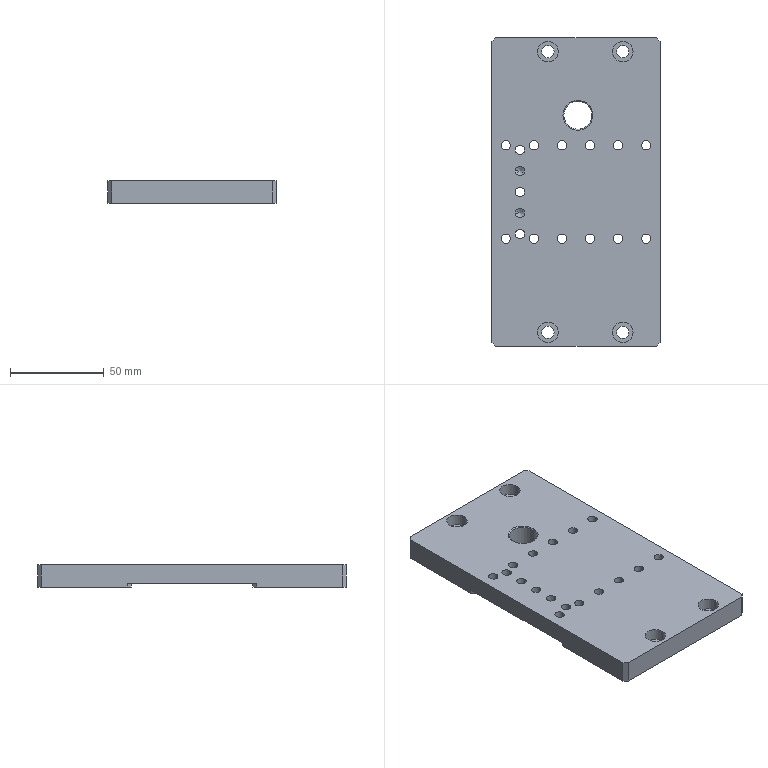NC program | NX | posted with a generic post | part box 90 x 165 x 12 mm
Whole program:
N10 G17 G21 G94 G90
(DRILLING , TOOL : D6A45)
N12 T01 M6
N14 G54
N16 G17 G0 G90 X157.5 Y60. S9500 M3
N18 G43 Z30. H1
N20 G94 G81 G98 Z-1. F250. R3.
N22 Y20.
N24 X107.5 Y7.5
N26 Y22.5
N28 Y37.5
N30 X123.5 Y44.
N32 X107.5 Y52.5
N34 Y67.5
N36 X105. Y75.
N38 X107.5 Y82.5
N40 X93.75 Y75.
N42 X82.5
N44 X71.25
N46 X57.5 Y82.5
N48 X60. Y75.
N50 X57.5 Y67.5
N52 Y52.5
N54 Y37.5
N56 Y22.5
N58 Y7.5
N60 X7.5 Y20.
N62 Y60.
N64 G80
N66 G0 X7.5 Y60. Z30.
N68 M5
(DRILLING_COPY , TOOL : 6.6ZT)
N70 T10 M6
N72 G54
N74 G17 G0 G90 X7.5 Y20. S2000 M3
N76 G43 Z30. H10
N78 G94 G83 G98 Z-14.483 F250. Q2. R3.
N80 Y60.
N82 X157.5
N84 Y20.
N86 G80
N88 G0 X157.5 Y20. Z30.
N90 M5
(DRILLING_COPY_COPY , TOOL : 5.0ZT)
N92 T17 M6
N94 G54
N96 G17 G0 G90 X107.5 Y7.5 S2000 M3
N98 G43 Z30. H17
N100 G94 G83 G98 Z-14.002 F250. Q2. R3.
N102 Y22.5
N104 Y37.5
N106 Y52.5
N108 Y67.5
N110 X105. Y75.
N112 X107.5 Y82.5
N114 X82.5 Y75.
N116 X57.5 Y82.5
N118 X60. Y75.
N120 X57.5 Y67.5
N122 Y52.5
N124 Y37.5
N126 Y22.5
N128 Y7.5
N130 G80
N132 G0 X57.5 Y7.5 Z30.
N134 M5
(ZLEVEL_PROFILE , TOOL : D10)
N136 T15 M6
N138 G54
N140 G17 G0 G90 X163.037 Y99.812 S9500 M3
N142 G43 Z30. H15
N144 Z2.
N146 G94 G1 Z-1. F1000.
N148 X162.629 Y98.29
N150 G3 X162.888 Y97.324 R1.
N152 G1 X167.249 Y92.964 F3000.
N154 X168.606 Y91.606
N156 G2 X170.1 Y88. R5.1
N158 G1 Y2.
N160 G2 X168.606 Y-1.606 R5.1
N162 G1 X166.674 Y-3.539
N164 G2 X166.056 Y-4.083 R6.519
N166 G1 X166.047 Y-4.165
N168 X162.888 Y-7.324
N170 G3 X162.629 Y-8.29 R1.
N172 G1 X163.037 Y-9.812
N174 Z2.
N176 G0 Z1.
N178 G1 Z-2. F1000.
N180 X162.629 Y-8.29
N182 G2 X162.888 Y-7.324 R1.
N184 G1 X166.047 Y-4.165 F3000.
N186 X166.056 Y-4.083
N188 G3 X166.674 Y-3.539 R6.519
N190 G1 X168.606 Y-1.606
N192 G3 X170.1 Y2. R5.1
N194 G1 Y88.
N196 G3 X168.606 Y91.606 R5.1
N198 G1 X167.249 Y92.964
N200 X162.888 Y97.324
N202 G2 X162.629 Y98.29 R1.
N204 G1 X163.037 Y99.812
N206 Z1.
N208 G0 Z0.
N210 G1 Z-3. F1000.
N212 X162.629 Y98.29
N214 G3 X162.888 Y97.324 R1.
N216 G1 X167.249 Y92.964 F3000.
N218 X168.606 Y91.606
N220 G2 X170.1 Y88. R5.1
N222 G1 Y2.
N224 G2 X168.606 Y-1.606 R5.1
N226 G1 X166.674 Y-3.539
N228 G2 X166.056 Y-4.083 R6.519
N230 G1 X166.047 Y-4.165
N232 X162.888 Y-7.324
N234 G3 X162.629 Y-8.29 R1.
N236 G1 X163.037 Y-9.812
N238 Z0.
N240 G0 Z-1.
N242 G1 Z-4. F1000.
N244 X162.629 Y-8.29
N246 G2 X162.888 Y-7.324 R1.
N248 G1 X166.047 Y-4.165 F3000.
N250 X166.056 Y-4.083
N252 G3 X166.674 Y-3.539 R6.519
N254 G1 X168.606 Y-1.606
N256 G3 X170.1 Y2. R5.1
N258 G1 Y88.
N260 G3 X168.606 Y91.606 R5.1
N262 G1 X167.249 Y92.964
N264 X162.888 Y97.324
N266 G2 X162.629 Y98.29 R1.
N268 G1 X163.037 Y99.812
N270 Z-1.
N272 G0 Z-2.
N274 G1 Z-5. F1000.
N276 X162.629 Y98.29
N278 G3 X162.888 Y97.324 R1.
N280 G1 X167.249 Y92.964 F3000.
N282 X168.606 Y91.606
N284 G2 X170.1 Y88. R5.1
N286 G1 Y2.
N288 G2 X168.606 Y-1.606 R5.1
N290 G1 X166.674 Y-3.539
N292 G2 X166.056 Y-4.083 R6.519
N294 G1 X166.047 Y-4.165
N296 X162.888 Y-7.324
N298 G3 X162.629 Y-8.29 R1.
N300 G1 X163.037 Y-9.812
N302 Z-2.
N304 G0 Z-3.
N306 G1 Z-6. F1000.
N308 X162.629 Y-8.29
N310 G2 X162.888 Y-7.324 R1.
N312 G1 X166.047 Y-4.165 F3000.
N314 X166.056 Y-4.083
N316 G3 X166.674 Y-3.539 R6.519
N318 G1 X168.606 Y-1.606
N320 G3 X170.1 Y2. R5.1
N322 G1 Y88.
N324 G3 X168.606 Y91.606 R5.1
N326 G1 X167.249 Y92.964
N328 X162.888 Y97.324
N330 G2 X162.629 Y98.29 R1.
N332 G1 X163.037 Y99.812
N334 Z-3.
N336 G0 Z-4.
N338 G1 Z-7. F1000.
N340 X162.629 Y98.29
N342 G3 X162.888 Y97.324 R1.
N344 G1 X167.249 Y92.964 F3000.
N346 X168.606 Y91.606
N348 G2 X170.1 Y88. R5.1
N350 G1 Y2.
N352 G2 X168.606 Y-1.606 R5.1
N354 G1 X166.674 Y-3.539
N356 G2 X166.056 Y-4.083 R6.519
N358 G1 X166.047 Y-4.165
N360 X162.888 Y-7.324
N362 G3 X162.629 Y-8.29 R1.
N364 G1 X163.037 Y-9.812
N366 Z-4.
N368 G0 Z-5.
N370 G1 Z-8. F1000.
N372 X162.629 Y-8.29
N374 G2 X162.888 Y-7.324 R1.
N376 G1 X166.047 Y-4.165 F3000.
N378 X166.056 Y-4.083
N380 G3 X166.674 Y-3.539 R6.519
N382 G1 X168.606 Y-1.606
N384 G3 X170.1 Y2. R5.1
N386 G1 Y88.
N388 G3 X168.606 Y91.606 R5.1
N390 G1 X167.249 Y92.964
N392 X162.888 Y97.324
N394 G2 X162.629 Y98.29 R1.
N396 G1 X163.037 Y99.812
N398 Z-5.
N400 G0 Z-6.
N402 G1 Z-9. F1000.
N404 X162.629 Y98.29
N406 G3 X162.888 Y97.324 R1.
N408 G1 X167.249 Y92.964 F3000.
N410 X168.606 Y91.606
N412 G2 X170.1 Y88. R5.1
N414 G1 Y2.
N416 G2 X168.606 Y-1.606 R5.1
N418 G1 X166.674 Y-3.539
N420 G2 X166.056 Y-4.083 R6.519
N422 G1 X166.047 Y-4.165
N424 X162.888 Y-7.324
N426 G3 X162.629 Y-8.29 R1.
N428 G1 X163.037 Y-9.812
N430 Z-6.
N432 G0 Z-7.
N434 G1 Z-10. F1000.
N436 X162.629 Y-8.29
N438 G2 X162.888 Y-7.324 R1.
N440 G1 X166.047 Y-4.165 F3000.
N442 X166.056 Y-4.083
N444 G3 X166.674 Y-3.539 R6.519
N446 G1 X168.606 Y-1.606
N448 G3 X170.1 Y2. R5.1
N450 G1 Y88.
N452 G3 X168.606 Y91.606 R5.1
N454 G1 X167.249 Y92.964
N456 X162.888 Y97.324
N458 G2 X162.629 Y98.29 R1.
N460 G1 X163.037 Y99.812
N462 Z-7.
N464 G0 Z-8.
N466 G1 Z-11. F1000.
N468 X162.629 Y98.29
N470 G3 X162.888 Y97.324 R1.
N472 G1 X167.249 Y92.964 F3000.
N474 X168.606 Y91.606
N476 G2 X170.1 Y88. R5.1
N478 G1 Y2.
N480 G2 X168.606 Y-1.606 R5.1
N482 G1 X166.674 Y-3.539
N484 G2 X166.056 Y-4.083 R6.519
N486 G1 X166.047 Y-4.165
N488 X162.888 Y-7.324
N490 G3 X162.629 Y-8.29 R1.
N492 G1 X163.037 Y-9.812
N494 Z-8.
N496 G0 Z-9.
N498 G1 Z-12. F1000.
N500 X162.629 Y-8.29
N502 G2 X162.888 Y-7.324 R1.
N504 G1 X166.047 Y-4.165 F3000.
N506 X166.056 Y-4.083
N508 G3 X166.674 Y-3.539 R6.519
N510 G1 X168.606 Y-1.606
N512 G3 X170.1 Y2. R5.1
N514 G1 Y88.
N516 G3 X168.606 Y91.606 R5.1
N518 G1 X167.249 Y92.964
N520 X162.888 Y97.324
N522 G2 X162.629 Y98.29 R1.
N524 G1 X163.037 Y99.812
N526 Z-9.
N528 G0 Z58.5
N530 X2.066 Y-9.873
N532 Z2.
N534 G1 Z-1. F1000.
N536 X2.465 Y-8.384
N538 G3 X2.206 Y-7.418 R1.
N540 G1 X-1.627 Y-3.585 F3000.
N542 X-2.9 Y-2.308
N544 X-3.018 Y-2.111
N546 G2 X-5.1 Y2. R5.1
N548 G1 Y88.
N550 G2 X-3.606 Y91.606 R5.1
N552 G1 X-1.606 Y93.606
N554 X2.106 Y97.318
N556 G3 X2.365 Y98.284 R1.
N558 G1 X1.957 Y99.805
N560 Z2.
N562 G0 Z1.
N564 G1 Z-2. F1000.
N566 X2.365 Y98.284
N568 G2 X2.106 Y97.318 R1.
N570 G1 X-1.606 Y93.606 F3000.
N572 X-3.606 Y91.606
N574 G3 X-5.1 Y88. R5.1
N576 G1 Y2.
N578 G3 X-3.018 Y-2.111 R5.1
N580 G1 X-2.9 Y-2.308
N582 X-1.627 Y-3.585
N584 X2.206 Y-7.418
N586 G2 X2.465 Y-8.384 R1.
N588 G1 X2.066 Y-9.873
N590 Z1.
N592 G0 Z0.
N594 G1 Z-3. F1000.
N596 X2.465 Y-8.384
N598 G3 X2.206 Y-7.418 R1.
N600 G1 X-1.627 Y-3.585 F3000.
N602 X-2.9 Y-2.308
N604 X-3.018 Y-2.111
N606 G2 X-5.1 Y2. R5.1
N608 G1 Y88.
N610 G2 X-3.606 Y91.606 R5.1
N612 G1 X-1.606 Y93.606
N614 X2.106 Y97.318
N616 G3 X2.365 Y98.284 R1.
N618 G1 X1.957 Y99.805
N620 Z0.
N622 G0 Z-1.
N624 G1 Z-4. F1000.
N626 X2.365 Y98.284
N628 G2 X2.106 Y97.318 R1.
N630 G1 X-1.606 Y93.606 F3000.
N632 X-3.606 Y91.606
N634 G3 X-5.1 Y88. R5.1
N636 G1 Y2.
N638 G3 X-3.018 Y-2.111 R5.1
N640 G1 X-2.9 Y-2.308
N642 X-1.627 Y-3.585
N644 X2.206 Y-7.418
N646 G2 X2.465 Y-8.384 R1.
N648 G1 X2.066 Y-9.873
N650 Z-1.
N652 G0 Z-2.
N654 G1 Z-5. F1000.
N656 X2.465 Y-8.384
N658 G3 X2.206 Y-7.418 R1.
N660 G1 X-1.627 Y-3.585 F3000.
N662 X-2.9 Y-2.308
N664 X-3.018 Y-2.111
N666 G2 X-5.1 Y2. R5.1
N668 G1 Y88.
N670 G2 X-3.606 Y91.606 R5.1
N672 G1 X-1.606 Y93.606
N674 X2.106 Y97.318
N676 G3 X2.365 Y98.284 R1.
N678 G1 X1.957 Y99.805
N680 Z-2.
N682 G0 Z-3.
N684 G1 Z-6. F1000.
N686 X2.365 Y98.284
N688 G2 X2.106 Y97.318 R1.
N690 G1 X-1.606 Y93.606 F3000.
N692 X-3.606 Y91.606
N694 G3 X-5.1 Y88. R5.1
N696 G1 Y2.
N698 G3 X-3.018 Y-2.111 R5.1
N700 G1 X-2.9 Y-2.308
N702 X-1.627 Y-3.585
N704 X2.206 Y-7.418
N706 G2 X2.465 Y-8.384 R1.
N708 G1 X2.066 Y-9.873
N710 Z-3.
N712 G0 Z-4.
N714 G1 Z-7. F1000.
N716 X2.465 Y-8.384
N718 G3 X2.206 Y-7.418 R1.
N720 G1 X-1.627 Y-3.585 F3000.
N722 X-2.9 Y-2.308
N724 X-3.018 Y-2.111
N726 G2 X-5.1 Y2. R5.1
N728 G1 Y88.
N730 G2 X-3.606 Y91.606 R5.1
N732 G1 X-1.606 Y93.606
N734 X2.106 Y97.318
N736 G3 X2.365 Y98.284 R1.
N738 G1 X1.957 Y99.805
N740 Z-4.
N742 G0 Z-5.
N744 G1 Z-8. F1000.
N746 X2.365 Y98.284
N748 G2 X2.106 Y97.318 R1.
N750 G1 X-1.606 Y93.606 F3000.
N752 X-3.606 Y91.606
N754 G3 X-5.1 Y88. R5.1
N756 G1 Y2.
N758 G3 X-3.018 Y-2.111 R5.1
N760 G1 X-2.9 Y-2.308
N762 X-1.627 Y-3.585
N764 X2.206 Y-7.418
N766 G2 X2.465 Y-8.384 R1.
N768 G1 X2.066 Y-9.873
N770 Z-5.
N772 G0 Z-6.
N774 G1 Z-9. F1000.
N776 X2.465 Y-8.384
N778 G3 X2.206 Y-7.418 R1.
N780 G1 X-1.627 Y-3.585 F3000.
N782 X-2.9 Y-2.308
N784 X-3.018 Y-2.111
N786 G2 X-5.1 Y2. R5.1
N788 G1 Y88.
N790 G2 X-3.606 Y91.606 R5.1
N792 G1 X-1.606 Y93.606
N794 X2.106 Y97.318
N796 G3 X2.365 Y98.284 R1.
N798 G1 X1.957 Y99.805
N800 Z-6.
N802 G0 Z-7.
N804 G1 Z-10. F1000.
N806 X2.365 Y98.284
N808 G2 X2.106 Y97.318 R1.
N810 G1 X-1.606 Y93.606 F3000.
N812 X-3.606 Y91.606
N814 G3 X-5.1 Y88. R5.1
N816 G1 Y2.
N818 G3 X-3.018 Y-2.111 R5.1
N820 G1 X-2.9 Y-2.308
N822 X-1.627 Y-3.585
N824 X2.206 Y-7.418
N826 G2 X2.465 Y-8.384 R1.
N828 G1 X2.066 Y-9.873
N830 Z-7.
N832 G0 Z-8.
N834 G1 Z-11. F1000.
N836 X2.465 Y-8.384
N838 G3 X2.206 Y-7.418 R1.
N840 G1 X-1.627 Y-3.585 F3000.
N842 X-2.9 Y-2.308
N844 X-3.018 Y-2.111
N846 G2 X-5.1 Y2. R5.1
N848 G1 Y88.
N850 G2 X-3.606 Y91.606 R5.1
N852 G1 X-1.606 Y93.606
N854 X2.106 Y97.318
N856 G3 X2.365 Y98.284 R1.
N858 G1 X1.957 Y99.805
N860 Z-8.
N862 G0 Z-9.
N864 G1 Z-12. F1000.
N866 X2.365 Y98.284
N868 G2 X2.106 Y97.318 R1.
N870 G1 X-1.606 Y93.606 F3000.
N872 X-3.606 Y91.606
N874 G3 X-5.1 Y88. R5.1
N876 G1 Y2.
N878 G3 X-3.018 Y-2.111 R5.1
N880 G1 X-2.9 Y-2.308
N882 X-1.627 Y-3.585
N884 X2.206 Y-7.418
N886 G2 X2.465 Y-8.384 R1.
N888 G1 X2.066 Y-9.873
N890 Z-9.
N892 G0 Z30.
N894 M5
(HOLE_MILLING , TOOL : D6)
N896 T12 M6
N898 G54
N900 G17 G0 G90 X7.5 Y60. S9500 M3
N902 G43 Z30. H12
N904 Z0.5
N906 G94 G3 X6.25 Y58.75 R1.25 F1500.
N908 X7.5 Y57.5 R1.25
N910 X7.5 Y57.5 Z-0.1 I0. J2.5
N912 X7.5 Y57.5 Z-0.7 I0. J2.5
N914 X7.5 Y57.5 Z-1.3 I0. J2.5
N916 X7.5 Y57.5 Z-1.9 I0. J2.5
N918 X7.5 Y57.5 Z-2.5 I0. J2.5
N920 X7.5 Y57.5 Z-3.1 I0. J2.5
N922 X7.5 Y57.5 Z-3.7 I0. J2.5
N924 X7.5 Y57.5 Z-4.3 I0. J2.5
N926 X7.5 Y57.5 Z-4.9 I0. J2.5
N928 X7.5 Y57.5 Z-5.5 I0. J2.5
N930 X7.5 Y57.5 Z-6.1 I0. J2.5
N932 X7.5 Y62.5 Z-6.4 I0. J2.5
N934 X5. Y60. R2.5
N936 X7.5 Y62.5 R-2.5
N938 X6.25 Y61.25 R1.25
N940 X7.5 Y60. R1.25
N942 G0 Z30.
N944 Y20.
N946 Z0.5
N948 G3 X6.25 Y18.75 R1.25
N950 X7.5 Y17.5 R1.25
N952 X7.5 Y17.5 Z-0.1 I0. J2.5
N954 X7.5 Y17.5 Z-0.7 I0. J2.5
N956 X7.5 Y17.5 Z-1.3 I0. J2.5
N958 X7.5 Y17.5 Z-1.9 I0. J2.5
N960 X7.5 Y17.5 Z-2.5 I0. J2.5
N962 X7.5 Y17.5 Z-3.1 I0. J2.5
N964 X7.5 Y17.5 Z-3.7 I0. J2.5
N966 X7.5 Y17.5 Z-4.3 I0. J2.5
N968 X7.5 Y17.5 Z-4.9 I0. J2.5
N970 X7.5 Y17.5 Z-5.5 I0. J2.5
N972 X7.5 Y17.5 Z-6.1 I0. J2.5
N974 X7.5 Y22.5 Z-6.4 I0. J2.5
N976 X5. Y20. R2.5
N978 X7.5 Y22.5 R-2.5
N980 X6.25 Y21.25 R1.25
N982 X7.5 Y20. R1.25
N984 G0 Z30.
N986 X123.5 Y44.
N988 Z0.5
N990 G3 X122.375 Y42.875 R1.125
N992 X123.5 Y41.75 R1.125
N994 X123.5 Y41.75 Z-0.1 I0. J2.25
N996 X123.5 Y41.75 Z-0.7 I0. J2.25
N998 X123.5 Y41.75 Z-1.3 I0. J2.25
N1000 X123.5 Y41.75 Z-1.9 I0. J2.25
N1002 X123.5 Y41.75 Z-2.5 I0. J2.25
N1004 X123.5 Y41.75 Z-3.1 I0. J2.25
N1006 X123.5 Y41.75 Z-3.7 I0. J2.25
N1008 X123.5 Y41.75 Z-4.3 I0. J2.25
N1010 X123.5 Y41.75 Z-4.9 I0. J2.25
N1012 X123.5 Y41.75 Z-5.5 I0. J2.25
N1014 X123.5 Y41.75 Z-6.1 I0. J2.25
N1016 X123.5 Y41.75 Z-6.7 I0. J2.25
N1018 X123.5 Y41.75 Z-7.3 I0. J2.25
N1020 X123.5 Y41.75 Z-7.9 I0. J2.25
N1022 X123.5 Y41.75 Z-8.5 I0. J2.25
N1024 X123.5 Y41.75 Z-9.1 I0. J2.25
N1026 X123.5 Y41.75 Z-9.7 I0. J2.25
N1028 X123.5 Y41.75 Z-10.3 I0. J2.25
N1030 X123.5 Y41.75 Z-10.9 I0. J2.25
N1032 X123.5 Y41.75 Z-11.5 I0. J2.25
N1034 X121.551 Y42.875 Z-12. R-2.25
N1036 X124.625 Y42.051 R2.25
N1038 X121.551 Y42.875 R-2.25
N1040 X123.088 Y42.463 R1.125
N1042 X123.5 Y44. R1.125
N1044 G0 Z0.5
N1046 G3 X121.25 Y41.75 R2.25
N1048 X123.5 Y39.5 R2.25
N1050 X123.5 Y39.5 Z-0.1 I0. J4.5
N1052 X123.5 Y39.5 Z-0.7 I0. J4.5
N1054 X123.5 Y39.5 Z-1.3 I0. J4.5
N1056 X123.5 Y39.5 Z-1.9 I0. J4.5
N1058 X123.5 Y39.5 Z-2.5 I0. J4.5
N1060 X123.5 Y39.5 Z-3.1 I0. J4.5
N1062 X123.5 Y39.5 Z-3.7 I0. J4.5
N1064 X123.5 Y39.5 Z-4.3 I0. J4.5
N1066 X123.5 Y39.5 Z-4.9 I0. J4.5
N1068 X123.5 Y39.5 Z-5.5 I0. J4.5
N1070 X123.5 Y39.5 Z-6.1 I0. J4.5
N1072 X123.5 Y39.5 Z-6.7 I0. J4.5
N1074 X123.5 Y39.5 Z-7.3 I0. J4.5
N1076 X123.5 Y39.5 Z-7.9 I0. J4.5
N1078 X123.5 Y39.5 Z-8.5 I0. J4.5
N1080 X123.5 Y39.5 Z-9.1 I0. J4.5
N1082 X123.5 Y39.5 Z-9.7 I0. J4.5
N1084 X123.5 Y39.5 Z-10.3 I0. J4.5
N1086 X123.5 Y39.5 Z-10.9 I0. J4.5
N1088 X123.5 Y39.5 Z-11.5 I0. J4.5
N1090 X119.603 Y41.75 Z-12. R-4.5
N1092 X125.75 Y40.103 R4.5
N1094 X119.603 Y41.75 R-4.5
N1096 X122.676 Y40.926 R2.25
N1098 X123.5 Y44. R2.25
N1100 G0 Z30.
N1102 X157.5 Y60.
N1104 Z0.5
N1106 G3 X156.25 Y58.75 R1.25
N1108 X157.5 Y57.5 R1.25
N1110 X157.5 Y57.5 Z-0.1 I0. J2.5
N1112 X157.5 Y57.5 Z-0.7 I0. J2.5
N1114 X157.5 Y57.5 Z-1.3 I0. J2.5
N1116 X157.5 Y57.5 Z-1.9 I0. J2.5
N1118 X157.5 Y57.5 Z-2.5 I0. J2.5
N1120 X157.5 Y57.5 Z-3.1 I0. J2.5
N1122 X157.5 Y57.5 Z-3.7 I0. J2.5
N1124 X157.5 Y57.5 Z-4.3 I0. J2.5
N1126 X157.5 Y57.5 Z-4.9 I0. J2.5
N1128 X157.5 Y57.5 Z-5.5 I0. J2.5
N1130 X157.5 Y57.5 Z-6.1 I0. J2.5
N1132 X157.5 Y62.5 Z-6.4 I0. J2.5
N1134 X155. Y60. R2.5
N1136 X157.5 Y62.5 R-2.5
N1138 X156.25 Y61.25 R1.25
N1140 X157.5 Y60. R1.25
N1142 G0 Z30.
N1144 Y20.
N1146 Z0.5
N1148 G3 X156.25 Y18.75 R1.25
N1150 X157.5 Y17.5 R1.25
N1152 X157.5 Y17.5 Z-0.1 I0. J2.5
N1154 X157.5 Y17.5 Z-0.7 I0. J2.5
N1156 X157.5 Y17.5 Z-1.3 I0. J2.5
N1158 X157.5 Y17.5 Z-1.9 I0. J2.5
N1160 X157.5 Y17.5 Z-2.5 I0. J2.5
N1162 X157.5 Y17.5 Z-3.1 I0. J2.5
N1164 X157.5 Y17.5 Z-3.7 I0. J2.5
N1166 X157.5 Y17.5 Z-4.3 I0. J2.5
N1168 X157.5 Y17.5 Z-4.9 I0. J2.5
N1170 X157.5 Y17.5 Z-5.5 I0. J2.5
N1172 X157.5 Y17.5 Z-6.1 I0. J2.5
N1174 X157.5 Y22.5 Z-6.4 I0. J2.5
N1176 X155. Y20. R2.5
N1178 X157.5 Y22.5 R-2.5
N1180 X156.25 Y21.25 R1.25
N1182 X157.5 Y20. R1.25
N1184 G0 Z30.
N1186 M5
(HOLE_MILLING_COPY , TOOL : D3)
N1188 T18 M6
N1190 G54
N1192 G17 G0 G90 X71.25 Y75. S9500 M3
N1194 G43 Z30. H18
N1196 Z0.5
N1198 G94 G3 X70.8 Y74.55 R0.45 F1200.
N1200 X71.25 Y74.1 R0.45
N1202 X71.25 Y74.1 Z0.3 I0. J0.9
N1204 X71.25 Y74.1 Z0.1 I0. J0.9
N1206 X71.25 Y74.1 Z-0.1 I0. J0.9
N1208 X71.25 Y74.1 Z-0.3 I0. J0.9
N1210 X71.25 Y74.1 Z-0.5 I0. J0.9
N1212 X71.25 Y74.1 Z-0.7 I0. J0.9
N1214 X71.25 Y74.1 Z-0.9 I0. J0.9
N1216 X71.25 Y74.1 Z-1.1 I0. J0.9
N1218 X71.25 Y74.1 Z-1.3 I0. J0.9
N1220 X71.25 Y74.1 Z-1.5 I0. J0.9
N1222 X71.25 Y74.1 Z-1.7 I0. J0.9
N1224 X71.25 Y74.1 Z-1.9 I0. J0.9
N1226 X71.25 Y74.1 Z-2.1 I0. J0.9
N1228 X71.25 Y74.1 Z-2.3 I0. J0.9
N1230 X71.25 Y74.1 Z-2.5 I0. J0.9
N1232 X71.25 Y74.1 Z-2.7 I0. J0.9
N1234 X71.25 Y74.1 Z-2.9 I0. J0.9
N1236 X71.25 Y74.1 Z-3.1 I0. J0.9
N1238 X71.25 Y74.1 Z-3.3 I0. J0.9
N1240 X71.25 Y74.1 Z-3.5 I0. J0.9
N1242 X71.25 Y74.1 Z-3.7 I0. J0.9
N1244 X71.25 Y74.1 Z-3.9 I0. J0.9
N1246 X71.25 Y74.1 Z-4.1 I0. J0.9
N1248 X71.25 Y74.1 Z-4.3 I0. J0.9
N1250 X71.25 Y74.1 Z-4.5 I0. J0.9
N1252 X71.25 Y74.1 Z-4.7 I0. J0.9
N1254 X71.25 Y74.1 Z-4.9 I0. J0.9
N1256 X71.25 Y74.1 Z-5.1 I0. J0.9
N1258 X71.25 Y74.1 Z-5.3 I0. J0.9
N1260 X71.25 Y74.1 Z-5.5 I0. J0.9
N1262 X71.25 Y74.1 Z-5.7 I0. J0.9
N1264 X71.25 Y74.1 Z-5.9 I0. J0.9
N1266 X71.25 Y75.9 Z-6. I0. J0.9
N1268 X70.35 Y75. R0.9
N1270 X71.25 Y75.9 R-0.9
N1272 X70.8 Y75.45 R0.45
N1274 X71.25 Y75. R0.45
N1276 G0 Z30.
N1278 X93.75
N1280 Z0.5
N1282 G3 X93.3 Y74.55 R0.45
N1284 X93.75 Y74.1 R0.45
N1286 X93.75 Y74.1 Z0.3 I0. J0.9
N1288 X93.75 Y74.1 Z0.1 I0. J0.9
N1290 X93.75 Y74.1 Z-0.1 I0. J0.9
N1292 X93.75 Y74.1 Z-0.3 I0. J0.9
N1294 X93.75 Y74.1 Z-0.5 I0. J0.9
N1296 X93.75 Y74.1 Z-0.7 I0. J0.9
N1298 X93.75 Y74.1 Z-0.9 I0. J0.9
N1300 X93.75 Y74.1 Z-1.1 I0. J0.9
N1302 X93.75 Y74.1 Z-1.3 I0. J0.9
N1304 X93.75 Y74.1 Z-1.5 I0. J0.9
N1306 X93.75 Y74.1 Z-1.7 I0. J0.9
N1308 X93.75 Y74.1 Z-1.9 I0. J0.9
N1310 X93.75 Y74.1 Z-2.1 I0. J0.9
N1312 X93.75 Y74.1 Z-2.3 I0. J0.9
N1314 X93.75 Y74.1 Z-2.5 I0. J0.9
N1316 X93.75 Y74.1 Z-2.7 I0. J0.9
N1318 X93.75 Y74.1 Z-2.9 I0. J0.9
N1320 X93.75 Y74.1 Z-3.1 I0. J0.9
N1322 X93.75 Y74.1 Z-3.3 I0. J0.9
N1324 X93.75 Y74.1 Z-3.5 I0. J0.9
N1326 X93.75 Y74.1 Z-3.7 I0. J0.9
N1328 X93.75 Y74.1 Z-3.9 I0. J0.9
N1330 X93.75 Y74.1 Z-4.1 I0. J0.9
N1332 X93.75 Y74.1 Z-4.3 I0. J0.9
N1334 X93.75 Y74.1 Z-4.5 I0. J0.9
N1336 X93.75 Y74.1 Z-4.7 I0. J0.9
N1338 X93.75 Y74.1 Z-4.9 I0. J0.9
N1340 X93.75 Y74.1 Z-5.1 I0. J0.9
N1342 X93.75 Y74.1 Z-5.3 I0. J0.9
N1344 X93.75 Y74.1 Z-5.5 I0. J0.9
N1346 X93.75 Y74.1 Z-5.7 I0. J0.9
N1348 X93.75 Y74.1 Z-5.9 I0. J0.9
N1350 X93.75 Y75.9 Z-6. I0. J0.9
N1352 X92.85 Y75. R0.9
N1354 X93.75 Y75.9 R-0.9
N1356 X93.3 Y75.45 R0.45
N1358 X93.75 Y75. R0.45
N1360 G0 Z30.
N1362 M5
(ZLEVEL_PROFILE_1 , TOOL : D10JING)
N1364 T14 M6
N1366 G54
N1368 G17 G0 G90 X166.668 Y95.962 S9500 M3
N1370 G43 Z30. H14
N1372 Z-10.5
N1374 G94 G1 Z-12. F1000.
N1376 X166.277 Y94.501
N1378 G3 X166.536 Y93.536 R1.
N1380 G1 X168.536 Y91.536 F1500.
N1382 G2 X170. Y88. R5.
N1384 G1 Y2.
N1386 G2 X168.536 Y-1.536 R5.
N1388 G1 X166.536 Y-3.536
N1390 G3 X166.277 Y-4.501 R1.
N1392 G1 X166.668 Y-5.962
N1394 Z-10.5
N1396 G0 Z30.
N1398 X-1.668
N1400 Z-10.5
N1402 G1 Z-12. F1000.
N1404 X-1.277 Y-4.501
N1406 G3 X-1.536 Y-3.536 R1.
N1408 G1 X-3.536 Y-1.536 F1500.
N1410 G2 X-5. Y2. R5.
N1412 G1 Y88.
N1414 G2 X-3.536 Y91.536 R5.
N1416 G1 X-1.536 Y93.536
N1418 G3 X-1.277 Y94.501 R1.
N1420 G1 X-1.668 Y95.962
N1422 Z-10.5
N1424 G0 Z30.
N1426 M5
(PLANAR_MILL_COPY , TOOL : D6A45)
N1428 T01 M6
N1430 G54
N1432 G17 G0 G90 X3.4 Y60.866 S9500 M3
N1434 G43 Z30. H1
N1436 Z0.5
N1438 G94 G1 Z-1. F1250.
N1440 G3 X2.9 Y60. R1.
N1442 X7.5 Y55.4 R4.6
N1444 X2.9 Y60. R-4.6
N1446 X3.4 Y59.134 R1.
N1448 G1 Z0.5
N1450 G0 Z30.
N1452 Y20.866
N1454 Z0.5
N1456 G1 Z-1.
N1458 G3 X2.9 Y20. R1.
N1460 X7.5 Y15.4 R4.6
N1462 X2.9 Y20. R-4.6
N1464 X3.4 Y19.134 R1.
N1466 G1 Z0.5
N1468 G0 Z30.
N1470 X56.634 Y6.4
N1472 Z0.5
N1474 G1 Z-1.
N1476 G3 X57.5 Y5.9 R1.
N1478 X59.1 Y7.5 R1.6
N1480 X57.5 Y5.9 R-1.6
N1482 X58.366 Y6.4 R1.
N1484 G1 Z0.5
N1486 G0 Z30.
N1488 X56.634 Y21.4
N1490 Z0.5
N1492 G1 Z-1.
N1494 G3 X57.5 Y20.9 R1.
N1496 X59.1 Y22.5 R1.6
N1498 X57.5 Y20.9 R-1.6
N1500 X58.366 Y21.4 R1.
N1502 G1 Z0.5
N1504 G0 Z30.
N1506 X56.634 Y36.4
N1508 Z0.5
N1510 G1 Z-1.
N1512 G3 X57.5 Y35.9 R1.
N1514 X59.1 Y37.5 R1.6
N1516 X57.5 Y35.9 R-1.6
N1518 X58.366 Y36.4 R1.
N1520 G1 Z0.5
N1522 G0 Z30.
N1524 X83.366 Y-1.4
N1526 Z0.5
N1528 G1 Z-1.
N1530 G3 X82.5 Y-0.9 R1.
N1532 G1 X2.
N1534 G2 X1.364 Y-0.636 R0.9
N1536 G1 X-0.636 Y1.364
N1538 G2 X-0.9 Y2. R0.9
N1540 G1 Y88.
N1542 G2 X-0.636 Y88.636 R0.9
N1544 G1 X1.364 Y90.636
N1546 G2 X2. Y90.9 R0.9
N1548 G1 X163.
N1550 G2 X163.636 Y90.636 R0.9
N1552 G1 X165.636 Y88.636
N1554 G2 X165.9 Y88. R0.9
N1556 G1 Y2.
N1558 G2 X165.636 Y1.364 R0.9
N1560 G1 X163.636 Y-0.636
N1562 G2 X163. Y-0.9 R0.9
N1564 G1 X82.5
N1566 G3 X81.634 Y-1.4 R1.
N1568 G1 Z0.5
N1570 G0 Z30.
N1572 X58.366 Y53.6
N1574 Z0.5
N1576 G1 Z-1.
N1578 G3 X57.5 Y54.1 R1.
N1580 X55.9 Y52.5 R1.6
N1582 X57.5 Y54.1 R-1.6
N1584 X56.634 Y53.6 R1.
N1586 G1 Z0.5
N1588 G0 Z30.
N1590 X58.366 Y68.6
N1592 Z0.5
N1594 G1 Z-1.
N1596 G3 X57.5 Y69.1 R1.
N1598 X55.9 Y67.5 R1.6
N1600 X57.5 Y69.1 R-1.6
N1602 X56.634 Y68.6 R1.
N1604 G1 Z0.5
N1606 G0 Z30.
N1608 X60.866 Y76.1
N1610 Z0.5
N1612 G1 Z-1.
N1614 G3 X60. Y76.6 R1.
N1616 X58.4 Y75. R1.6
N1618 X60. Y76.6 R-1.6
N1620 X59.134 Y76.1 R1.
N1622 G1 Z0.5
N1624 G0 Z30.
N1626 X58.366 Y83.6
N1628 Z0.5
N1630 G1 Z-1.
N1632 G3 X57.5 Y84.1 R1.
N1634 X55.9 Y82.5 R1.6
N1636 X57.5 Y84.1 R-1.6
N1638 X56.634 Y83.6 R1.
N1640 G1 Z0.5
N1642 G0 Z30.
N1644 X72.116 Y76.1
N1646 Z0.5
N1648 G1 Z-1.
N1650 G3 X71.25 Y76.6 R1.
N1652 X69.65 Y75. R1.6
N1654 X71.25 Y76.6 R-1.6
N1656 X70.384 Y76.1 R1.
N1658 G1 Z0.5
N1660 G0 Z30.
N1662 X83.366
N1664 Z0.5
N1666 G1 Z-1.
N1668 G3 X82.5 Y76.6 R1.
N1670 X80.9 Y75. R1.6
N1672 X82.5 Y76.6 R-1.6
N1674 X81.634 Y76.1 R1.
N1676 G1 Z0.5
N1678 G0 Z30.
N1680 X94.616
N1682 Z0.5
N1684 G1 Z-1.
N1686 G3 X93.75 Y76.6 R1.
N1688 X92.15 Y75. R1.6
N1690 X93.75 Y76.6 R-1.6
N1692 X92.884 Y76.1 R1.
N1694 G1 Z0.5
N1696 G0 Z30.
N1698 X108.366 Y83.6
N1700 Z0.5
N1702 G1 Z-1.
N1704 G3 X107.5 Y84.1 R1.
N1706 X105.9 Y82.5 R1.6
N1708 X107.5 Y84.1 R-1.6
N1710 X106.634 Y83.6 R1.
N1712 G1 Z0.5
N1714 G0 Z30.
N1716 X105.866 Y76.1
N1718 Z0.5
N1720 G1 Z-1.
N1722 G3 X105. Y76.6 R1.
N1724 X103.4 Y75. R1.6
N1726 X105. Y76.6 R-1.6
N1728 X104.134 Y76.1 R1.
N1730 G1 Z0.5
N1732 G0 Z30.
N1734 X108.366 Y68.6
N1736 Z0.5
N1738 G1 Z-1.
N1740 G3 X107.5 Y69.1 R1.
N1742 X105.9 Y67.5 R1.6
N1744 X107.5 Y69.1 R-1.6
N1746 X106.634 Y68.6 R1.
N1748 G1 Z0.5
N1750 G0 Z30.
N1752 X108.366 Y53.6
N1754 Z0.5
N1756 G1 Z-1.
N1758 G3 X107.5 Y54.1 R1.
N1760 X105.9 Y52.5 R1.6
N1762 X107.5 Y54.1 R-1.6
N1764 X106.634 Y53.6 R1.
N1766 G1 Z0.5
N1768 G0 Z30.
N1770 Y36.4
N1772 Z0.5
N1774 G1 Z-1.
N1776 G3 X107.5 Y35.9 R1.
N1778 X109.1 Y37.5 R1.6
N1780 X107.5 Y35.9 R-1.6
N1782 X108.366 Y36.4 R1.
N1784 G1 Z0.5
N1786 G0 Z30.
N1788 X106.634 Y21.4
N1790 Z0.5
N1792 G1 Z-1.
N1794 G3 X107.5 Y20.9 R1.
N1796 X109.1 Y22.5 R1.6
N1798 X107.5 Y20.9 R-1.6
N1800 X108.366 Y21.4 R1.
N1802 G1 Z0.5
N1804 G0 Z30.
N1806 X106.634 Y6.4
N1808 Z0.5
N1810 G1 Z-1.
N1812 G3 X107.5 Y5.9 R1.
N1814 X109.1 Y7.5 R1.6
N1816 X107.5 Y5.9 R-1.6
N1818 X108.366 Y6.4 R1.
N1820 G1 Z0.5
N1822 G0 Z30.
N1824 X161.6 Y19.134
N1826 Z0.5
N1828 G1 Z-1.
N1830 G3 X162.1 Y20. R1.
N1832 X157.5 Y24.6 R4.6
N1834 X162.1 Y20. R-4.6
N1836 X161.6 Y20.866 R1.
N1838 G1 Z0.5
N1840 G0 Z30.
N1842 Y59.134
N1844 Z0.5
N1846 G1 Z-1.
N1848 G3 X162.1 Y60. R1.
N1850 X157.5 Y64.6 R4.6
N1852 X162.1 Y60. R-4.6
N1854 X161.6 Y60.866 R1.
N1856 G1 Z0.5
N1858 G0 Z30.
(PLANAR_MILL_COPY_COPY , TOOL : D6A45)
N1860 X124.366 Y50.
N1862 Z0.
N1864 G1 Z-1.5
N1866 G3 X123.5 Y50.5 R1.
N1868 X117. Y44. R6.5
N1870 X123.5 Y50.5 R-6.5
N1872 X122.634 Y50. R1.
N1874 G1 Z0.
N1876 G0 Z30.
N1878 M5
(18刀补 , TOOL : D3)
N1880 T18 M6
N1882 G54
N1884 G17 G0 G90 X71.25 Y75. S9500 M3
N1886 G43 Z30. H18
N1888 Z0.5
N1890 G41 G94 G1 X71.15 Y74.996 F1200. D18
N1892 G3 X71.25 Y74.05 R0.478
N1894 X71.25 Y74.05 Z-1.5 I0. J0.95
N1896 X71.25 Y74.05 Z-3.5 I0. J0.95
N1898 X71.25 Y74.05 Z-5.5 I0. J0.95
N1900 X72.2 Y75. Z-6. R0.95
N1902 X71.25 Y75.95 R0.95
N1904 X72.2 Y75. R-0.95
N1906 X71.254 Y75.1 R0.478
N1908 G40
N1910 G1 X71.25 Y75.
N1912 G0 Z30.
N1914 X93.75
N1916 Z0.5
N1918 G41 G1 X93.65 Y74.996
N1920 G3 X93.75 Y74.05 R0.478
N1922 X93.75 Y74.05 Z-1.5 I0. J0.95
N1924 X93.75 Y74.05 Z-3.5 I0. J0.95
N1926 X93.75 Y74.05 Z-5.5 I0. J0.95
N1928 X94.7 Y75. Z-6. R0.95
N1930 X93.75 Y75.95 R0.95
N1932 X94.7 Y75. R-0.95
N1934 X93.754 Y75.1 R0.478
N1936 G40
N1938 G1 X93.75 Y75.
N1940 G0 Z30.
N1942 M5
N1944 M2